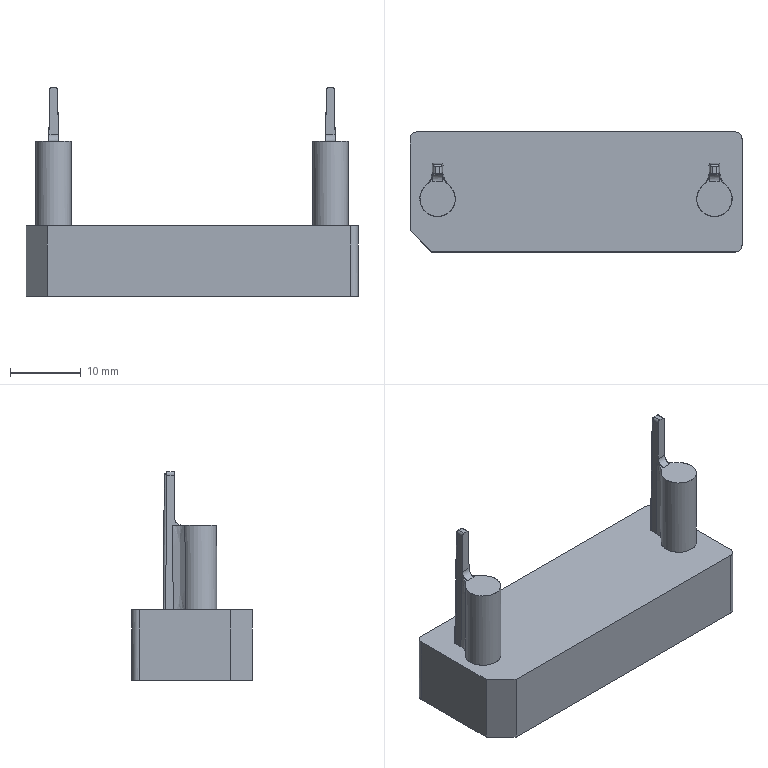NC program | PowerMill | posted with a generic post | part box 47 x 17 x 29.578 mm
Lines 10016 to 10829 of 182382:
N10113 M6
N10114 S8500 M03
N10115 G00 G90 X0.0 Y0.0
N10116 G43 Z11.798 H3
N10117
N10118 G05 P10000 R8
N10119 X-7.8085 Y4.5718
N10120 Z-6.78
N10121 G01 Z-7.98 F360.0
N10122 X-12.585 Y2.3334 F600.0
N10123 G03 X-12.6868 Y1.9988 I0.4982 J-0.3345
N10124 G01 X-12.6961 Y1.1864
N10125 X-12.7289 Y0.8046
N10126 G02 X-12.8666 Y0.0409 I-7.2156 J0.9069
N10127 G01 X-12.9741 Y-0.341
N10128 X-13.0825 Y-0.6564
N10129 X-13.2699 Y-1.1046
N10130 X-13.4635 Y-1.4865
N10131 X-13.6926 Y-1.8683
N10132 X-13.8754 Y-2.1353
N10133 X-14.0648 Y-2.3837
N10134 X-14.2757 Y-2.632
N10135 X-14.6682 Y-3.034
N10136 X-15.0918 Y-3.3957
N10137 X-15.4611 Y-3.6634
N10138 X-15.8576 Y-3.9074
N10139 X-16.3531 Y-4.1594
N10140 X-16.7 Y-4.3044
N10141 X-17.0469 Y-4.4264
N10142 X-17.4433 Y-4.5379
N10143 X-17.8398 Y-4.6218
N10144 X-18.2362 Y-4.6794
N10145 X-18.6326 Y-4.7112
N10146 X-19.0291 Y-4.7179
N10147 X-19.4255 Y-4.7001
N10148 X-20.2184 Y-4.7187
N10149 X-20.6148 Y-4.7083
N10150 X-21.0113 Y-4.6732
N10151 X-21.4077 Y-4.612
N10152 X-21.8041 Y-4.5248
N10153 X-22.2006 Y-4.4091
N10154 X-22.597 Y-4.2645
N10155 X-22.8425 Y-4.1594
N10156 X-23.3899 Y-3.8775
N10157 X-23.7469 Y-3.6541
N10158 X-24.1828 Y-3.333
N10159 X-24.5513 Y-3.0108
N10160 X-24.9757 Y-2.5686
N10161 X-25.2581 Y-2.2185
N10162 X-25.503 Y-1.8683
N10163 X-25.7685 Y-1.4179
N10164 X-25.9249 Y-1.1046
N10165 X-26.0874 Y-0.7228
N10166 X-26.2215 Y-0.341
N10167 X-26.3282 Y0.0409
N10168 X-26.4089 Y0.4227
N10169 X-26.4659 Y0.8046
N10170 X-26.4987 Y1.1864
N10171 X-26.5137 Y2.414
N10172 X-26.5306 Y2.4948
N10173 G00 Z3.9981
N10174 G01 X-19.1136 Y-9.0107 F10000.0
N10175 G00 Z0.7981
N10176 G01 Z-0.4019 F360.0
N10177 X-19.147 Y-3.7358 F600.0
N10178 Y0.5589
N10179 G03 X-17.8411 Y1.8648 I0.0 J1.3059
N10180 G03 X-20.4529 I-1.3059 J0.0
N10181 G03 X-19.147 Y0.5589 I1.3059 J0.0
N10182 G01 Y-3.7358
N10183 G00 Z5.6117
N10184 G01 X31.4193 Y4.5014 F10000.0
N10185 G00 Z-6.78
N10186 G01 Z-7.98 F360.0
N10187 X26.616 Y2.3211 F600.0
N10188 G03 X26.508 Y1.9777 I0.492 J-0.3434
N10189 G01 X26.4987 Y1.1864
N10190 X26.4662 Y0.8046
N10191 X26.4089 Y0.4227
N10192 X26.3278 Y0.0409
N10193 X26.2215 Y-0.341
N10194 X26.0874 Y-0.7228
N10195 X25.9249 Y-1.1046
N10196 X25.7685 Y-1.4179
N10197 X25.503 Y-1.8683
N10198 X25.2581 Y-2.2185
N10199 X24.9199 Y-2.632
N10200 X24.5513 Y-3.0108
N10201 X24.1038 Y-3.3957
N10202 X23.7469 Y-3.6541
N10203 X23.3899 Y-3.8775
N10204 X22.8425 Y-4.1594
N10205 X22.597 Y-4.2645
N10206 X22.2006 Y-4.4091
N10207 X21.8041 Y-4.5248
N10208 X21.4077 Y-4.612
N10209 X21.0113 Y-4.6732
N10210 X20.6148 Y-4.7083
N10211 X20.2184 Y-4.7187
N10212 X19.4255 Y-4.7001
N10213 X19.0291 Y-4.7179
N10214 X18.6326 Y-4.7112
N10215 X18.2362 Y-4.6794
N10216 X17.8398 Y-4.6218
N10217 X17.4433 Y-4.5379
N10218 X17.0469 Y-4.4264
N10219 X16.7 Y-4.3044
N10220 X16.254 Y-4.1139
N10221 X15.8576 Y-3.9074
N10222 X15.4611 Y-3.6634
N10223 X15.0918 Y-3.3957
N10224 X14.6682 Y-3.034
N10225 X14.2757 Y-2.632
N10226 X14.0648 Y-2.3837
N10227 X13.8754 Y-2.1353
N10228 X13.6926 Y-1.8683
N10229 X13.4633 Y-1.4865
N10230 X13.2699 Y-1.1046
N10231 X13.0825 Y-0.6564
N10232 X12.9741 Y-0.341
N10233 X12.8672 Y0.0409
N10234 X12.7859 Y0.4227
N10235 X12.7288 Y0.8046
N10236 X12.6961 Y1.1864
N10237 X12.6818 Y2.4218
N10238 X12.6664 Y2.499
N10239 G00 Z3.9981
N10240 G01 X19.0662 Y14.103 F10000.0
N10241 G00 Z0.7981
N10242 G01 Z-0.4019 F360.0
N10243 X19.1174 Y8.8282 F600.0
N10244 Y4.566
N10245 G03 X17.7611 Y3.2097 I0.0 J-1.3563
N10246 G03 X20.4737 I1.3563 J0.0
N10247 G03 X19.1174 Y4.566 I-1.3563 J0.0
N10248 G01 Y8.8282
N10249 G00 Z11.798
N10250 G05 P0
N10251 (---------------)
N10252 ( END TOOLPATH : 粗公基准台01-平坦面偏置-D10 )
N10253 (---------------)
N10254 ( START TOOLPATH : 粗公基准台01-基准面偏置-D10 )
N10255 (---------------)
N10256 G00 X0.0 Y0.0 Z9.7981
N10257 G05 P10000 R8
N10258 X34.035 Y-0.9466
N10259 Z-18.58
N10260 G01 Z-19.78 F360.0
N10261 X28.76 F600.0
N10262 X27.3406 Y-0.9827
N10263 X27.3456 Y-1.1792
N10264 X27.2856 Y-1.9654
N10265 X27.1818 Y-2.5788
N10266 X27.1433 Y-2.7515
N10267 X26.9148 Y-3.5376
N10268 X26.7644 Y-3.9307
N10269 X26.5916 Y-4.3238
N10270 X26.3939 Y-4.7084
N10271 X26.1577 Y-5.1099
N10272 X25.8999 Y-5.4942
N10273 X25.5922 Y-5.8961
N10274 X25.2434 Y-6.2891
N10275 X24.8181 Y-6.7122
N10276 X24.4242 Y-7.0479
N10277 X24.0302 Y-7.3409
N10278 X23.8417 Y-7.4684
N10279 X23.2424 Y-7.8238
N10280 X22.8484 Y-8.0197
N10281 X22.4545 Y-8.1885
N10282 X22.2791 Y-8.2545
N10283 X21.6666 Y-8.4526
N10284 X21.2727 Y-8.5502
N10285 X20.8787 Y-8.6268
N10286 X20.4848 Y-8.6832
N10287 X20.0909 Y-8.719
N10288 X19.6969 Y-8.7333
N10289 X19.303 Y-8.7267
N10290 X18.909 Y-8.7036
N10291 X18.5151 Y-8.6576
N10292 X18.1212 Y-8.5924
N10293 X17.7272 Y-8.5055
N10294 X17.3333 Y-8.3955
N10295 X16.9155 Y-8.2545
N10296 X16.5335 Y-8.101
N10297 X16.1515 Y-7.9259
N10298 X15.7575 Y-7.7152
N10299 X15.3528 Y-7.4684
N10300 X14.9643 Y-7.1962
N10301 X14.5757 Y-6.8841
N10302 X14.3441 Y-6.6822
N10303 X14.0524 Y-6.3974
N10304 X13.7878 Y-6.1126
N10305 X13.6032 Y-5.8961
N10306 X13.3017 Y-5.503
N10307 X13.0369 Y-5.1099
N10308 X12.789 Y-4.6862
N10309 X12.6037 Y-4.3238
N10310 X12.4309 Y-3.9307
N10311 X12.2798 Y-3.5376
N10312 X12.2121 Y-3.3311
N10313 X12.0513 Y-2.7515
N10314 X11.9097 Y-1.9654
N10315 X11.8497 Y-1.1792
N10316 X11.8697 Y-0.3931
N10317 X11.9098 Y0.0
N10318 X11.9705 Y0.3931
N10319 X12.1552 Y1.1792
N10320 X12.2121 Y1.3642
N10321 X12.4306 Y1.9654
N10322 X12.513 Y2.1692
N10323 G03 X12.5857 Y2.5625 I-0.9272 J0.3747
N10324 G01 X12.5822 Y3.5376
N10325 X12.6014 Y4.3238
N10326 X12.6446 Y4.7169
N10327 X12.713 Y5.1099
N10328 X12.808 Y5.503
N10329 X12.93 Y5.8961
N10330 X13.0 Y6.0872
N10331 X13.2531 Y6.6822
N10332 X13.4634 Y7.0753
N10333 X13.7109 Y7.4684
N10334 X14.048 Y7.9159
N10335 X14.3411 Y8.2545
N10336 X14.5757 Y8.4956
N10337 X14.8962 Y8.7867
N10338 X15.2166 Y9.0406
N10339 X15.3636 Y9.1466
N10340 X15.7575 Y9.3994
N10341 X16.1515 Y9.6195
N10342 X16.5931 Y9.8268
N10343 X16.9394 Y9.9611
N10344 X17.3333 Y10.0861
N10345 X17.7272 Y10.1838
N10346 X18.1212 Y10.2565
N10347 X18.5151 Y10.3082
N10348 X18.909 Y10.3341
N10349 X20.0909 Y10.3381
N10350 X20.4848 Y10.324
N10351 X20.8787 Y10.2851
N10352 X21.2727 Y10.2216
N10353 X21.6666 Y10.1377
N10354 X22.0606 Y10.0266
N10355 X22.4545 Y9.8867
N10356 X22.9219 Y9.6805
N10357 X23.2424 Y9.512
N10358 X23.6105 Y9.293
N10359 X24.0302 Y9.0023
N10360 X24.4242 Y8.6773
N10361 X24.8535 Y8.2545
N10362 X25.1915 Y7.8614
N10363 X25.4837 Y7.4684
N10364 X25.606 Y7.2826
N10365 X25.7846 Y6.9824
N10366 X25.9415 Y6.6822
N10367 X26.1168 Y6.2891
N10368 X26.2646 Y5.8961
N10369 X26.3939 Y5.4777
N10370 X26.4824 Y5.1099
N10371 X26.5506 Y4.7169
N10372 X26.5939 Y4.3238
N10373 X26.6132 Y3.5376
N10374 X26.6119 Y2.547
N10375 G03 X26.6943 Y2.1276 I0.9997 J-0.0213
N10376 G01 X26.7647 Y1.9654
N10377 X27.0394 Y1.1792
N10378 G02 X27.2241 Y0.3931 I-7.7339 J-2.2314
N10379 G01 X27.3256 Y-0.3931
N10380 X27.3406 Y-0.9827
N10381 X28.76 Y-0.9466
N10382 G00 Z2.8214
N10383 G01 X-34.0345 Y-1.1435 F10000.0
N10384 G00 Z-18.58
N10385 G01 Z-19.78 F360.0
N10386 X-28.7595 Y-1.1432 F600.0
N10387 X-27.3456 Y-1.1792
N10388 X-27.3256 Y-0.3931
N10389 X-27.2241 Y0.3931
N10390 X-27.1398 Y0.788
N10391 X-27.0394 Y1.1792
N10392 X-26.7647 Y1.9654
N10393 X-26.6824 Y2.1688
N10394 G03 X-26.6096 Y2.563 I-0.9269 J0.3751
N10395 G01 X-26.6132 Y3.5376
N10396 X-26.5939 Y4.3238
N10397 X-26.5503 Y4.7169
N10398 X-26.4824 Y5.1099
N10399 X-26.3939 Y5.4777
N10400 X-26.2646 Y5.8961
N10401 X-26.1172 Y6.2891
N10402 X-25.9415 Y6.6822
N10403 X-25.7847 Y6.9824
N10404 X-25.606 Y7.2826
N10405 X-25.4837 Y7.4684
N10406 X-25.1918 Y7.8614
N10407 X-24.8181 Y8.2929
N10408 X-24.4242 Y8.6773
N10409 X-23.9787 Y9.0406
N10410 X-23.6105 Y9.293
N10411 X-23.2424 Y9.512
N10412 X-22.9219 Y9.6805
N10413 X-22.4545 Y9.8867
N10414 X-22.0606 Y10.0266
N10415 X-21.6666 Y10.1377
N10416 X-21.2727 Y10.2216
N10417 X-20.8787 Y10.2851
N10418 X-20.4848 Y10.324
N10419 X-20.0909 Y10.3381
N10420 X-18.909 Y10.3341
N10421 X-18.5151 Y10.3082
N10422 X-18.1212 Y10.2565
N10423 X-17.7272 Y10.1838
N10424 X-17.3333 Y10.0861
N10425 X-16.9394 Y9.9611
N10426 X-16.5931 Y9.8268
N10427 X-16.1515 Y9.6195
N10428 X-15.7575 Y9.3994
N10429 X-15.3636 Y9.1466
N10430 X-15.2166 Y9.0406
N10431 X-14.8962 Y8.7867
N10432 X-14.5757 Y8.4956
N10433 X-14.3411 Y8.2545
N10434 X-14.0477 Y7.9159
N10435 X-13.7109 Y7.4684
N10436 X-13.4632 Y7.0753
N10437 X-13.2531 Y6.6822
N10438 X-13.0 Y6.0872
N10439 X-12.93 Y5.8961
N10440 X-12.8077 Y5.503
N10441 X-12.713 Y5.1099
N10442 X-12.6445 Y4.7169
N10443 X-12.6014 Y4.3238
N10444 X-12.5822 Y3.5376
N10445 X-12.583 Y2.545
N10446 G03 X-12.5014 Y2.1293 I0.9998 J-0.0195
N10447 G01 X-12.4306 Y1.9654
N10448 X-12.2121 Y1.3642
N10449 X-12.1552 Y1.1792
N10450 X-11.9705 Y0.3931
N10451 X-11.869 Y-0.4193
N10452 X-2.2734 Y0.1437
N10453 G02 X-2.2792 Y-2.1608 I-18.8247 J-1.1045
N10454 G01 X-2.3297 Y-2.9522
N10455 G03 X-1.2091 Y-4.1467 I1.1208 J-0.0714
N10456 G01 X1.2114 Y-4.147
N10457 G03 X2.332 Y-2.9567 I0.0001 J1.1225
N10458 G01 X2.276 Y-2.0314
N10459 G02 X2.295 Y0.3071 I17.0305 J1.031
N10460 G01 X2.3313 Y0.7203
N10461 X2.641 Y2.8499
N10462 G03 X1.5166 Y4.1496 I-1.1244 J0.1635
N10463 G01 X-1.5162
N10464 G03 X-2.6206 Y2.825 I0.0 J-1.1226
N10465 G01 X-2.5487 Y2.4317
N10466 G02 X-2.2734 Y0.1437 I-18.5495 J-3.3925
N10467 G01 X-7.0704 Y-0.1377
N10468 G03 X-7.198 Y1.0035 I-12.6157 J-0.8323
N10469 G01 X-7.9137 Y5.5324
N10470 G03 X-8.2698 Y7.082 I-11.3678 J-1.7964
N10471 G01 X-8.4987 Y7.8355
N10472 G02 X-7.6689 Y8.9549 I0.8298 J0.2521
N10473 G01 X7.6689
N10474 G02 X8.4947 Y7.8198 I0.0 J-0.8679
N10475 G01 X8.3902 Y7.497
N10476 G03 X7.8975 Y5.4331 I12.8607 J-4.1612
N10477 G01 X7.1542 Y0.6691
N10478 X7.1051 Y0.2146
N10479 G03 X8.7248 Y-7.2436 I12.424 J-1.2068
N10480 G01 X9.0865 Y-7.8687
N10481 G02 X8.461 Y-8.9532 I-0.6254 J-0.3619
N10482 G01 X-8.4587 Y-8.951
N10483 G02 X-9.0747 Y-7.8513 I0.0001 J0.7224
N10484 G01 X-8.9039 Y-7.5725
N10485 G03 X-7.0704 Y-0.1377 I-10.7821 J6.6025
N10486 G01 X-11.869 Y-0.4193
N10487 X-11.8497 Y-1.1792
N10488 X-11.9097 Y-1.9654
N10489 X-12.0513 Y-2.7515
N10490 X-12.2121 Y-3.3311
N10491 X-12.2798 Y-3.5376
N10492 X-12.4306 Y-3.9307
N10493 X-12.6037 Y-4.3238
N10494 X-12.7884 Y-4.6862
N10495 X-13.0369 Y-5.1099
N10496 X-13.3014 Y-5.503
N10497 X-13.6032 Y-5.8961
N10498 X-13.7878 Y-6.1126
N10499 X-14.0517 Y-6.3959
N10500 X-14.3441 Y-6.6822
N10501 X-14.5757 Y-6.8872
N10502 X-14.9658 Y-7.1969
N10503 X-15.3528 Y-7.4684
N10504 X-15.7575 Y-7.7152
N10505 X-16.1515 Y-7.9259
N10506 X-16.5362 Y-8.1025
N10507 X-16.9155 Y-8.2545
N10508 X-17.3333 Y-8.3955
N10509 X-17.7272 Y-8.5055
N10510 X-18.1212 Y-8.5924
N10511 X-18.5151 Y-8.6576
N10512 X-18.909 Y-8.7036
N10513 X-19.303 Y-8.7267
N10514 X-19.6969 Y-8.7333
N10515 X-20.0909 Y-8.719
N10516 X-20.4848 Y-8.6832
N10517 X-20.8787 Y-8.6268
N10518 X-21.2727 Y-8.5502
N10519 X-21.6666 Y-8.4526
N10520 X-22.2791 Y-8.2545
N10521 X-22.4545 Y-8.1885
N10522 X-22.8484 Y-8.0197
N10523 X-23.2424 Y-7.8238
N10524 X-23.8417 Y-7.4684
N10525 X-24.0302 Y-7.3409
N10526 X-24.4242 Y-7.0479
N10527 X-24.8181 Y-6.7122
N10528 X-25.0368 Y-6.5048
N10529 X-25.2472 Y-6.2891
N10530 X-25.5922 Y-5.8961
N10531 X-25.9 Y-5.4942
N10532 X-26.1577 Y-5.1099
N10533 X-26.3939 Y-4.7084
N10534 X-26.5916 Y-4.3238
N10535 X-26.7651 Y-3.9307
N10536 X-26.9148 Y-3.5376
N10537 X-27.1433 Y-2.7515
N10538 X-27.1818 Y-2.5788
N10539 X-27.2856 Y-1.9654
N10540 X-27.3456 Y-1.1792
N10541 X-28.7595 Y-1.1432
N10542 G00 Z9.7981
N10543 G05 P0
N10544 (---------------)
N10545 ( END TOOLPATH : 粗公基准台01-基准面偏置-D10 )
N10546 (---------------)
N10547 ( START TOOLPATH : 粗公基准台01-基准台侧光-D10 )
N10548 (---------------)
N10549 G00 X0.0 Y0.0 Z9.7981
N10550 G05 P10000 R8
N10551 X28.6685 Y-16.7036
N10552 Z-28.48
N10553 G01 Z-29.68 F360.0
N10554 G03 X25.8678 Y-12.5616 I-1.4004 J2.071 F600.0
N10555 G01 X25.8378 Y-12.5819
N10556 X25.8361 Y-12.583
N10557 X25.8344 Y-12.584
N10558 X25.5196 Y-12.7745
N10559 X25.5174 Y-12.7757
N10560 X25.5152 Y-12.7769
N10561 X25.0683 Y-13.0105
N10562 X25.0651 Y-13.0121
N10563 X25.0619 Y-13.0135
N10564 X24.6149 Y-13.1993
N10565 X24.6121 Y-13.2005
N10566 X24.6091 Y-13.2015
N10567 X24.1622 Y-13.3481
N10568 X24.1592 Y-13.349
N10569 X24.1561 Y-13.3498
N10570 X23.7092 Y-13.4585
N10571 X23.707 Y-13.459
N10572 X23.7049 Y-13.4594
N10573 X23.5507 Y-13.4882
N10574 X23.5493 Y-13.4885
N10575 X23.5479 Y-13.4887
N10576 X23.2551 Y-13.5326
N10577 X23.2526 Y-13.533
N10578 X23.25 Y-13.5333
N10579 X22.803 Y-13.571
N10580 X22.8004 Y-13.5712
N10581 X22.7978
N10582 X22.3509 Y-13.58
N10583 X22.3501
N10584 X22.3493
N10585 X-20.5613 Y-13.5796
N10586 X-20.5636
N10587 X-20.5659 Y-13.5795
N10588 X-21.0129 Y-13.554
N10589 X-21.0164 Y-13.5537
N10590 X-21.02 Y-13.5532
N10591 X-21.4583 Y-13.4887
N10592 X-21.4619 Y-13.4881
N10593 X-21.4655 Y-13.4873
N10594 X-21.9211 Y-13.3771
N10595 X-21.9247 Y-13.3762
N10596 X-21.9283 Y-13.375
N10597 X-22.3753 Y-13.2211
N10598 X-22.3788 Y-13.2198
N10599 X-22.3822 Y-13.2184
N10600 X-22.7879 Y-13.0355
N10601 X-22.7916 Y-13.0338
N10602 X-22.7951 Y-13.0318
N10603 X-23.2833 Y-12.7495
N10604 X-23.2862 Y-12.7478
N10605 X-23.2891 Y-12.7459
N10606 X-23.5249 Y-12.5812
N10607 X-23.5267 Y-12.5799
N10608 X-23.5285 Y-12.5785
N10609 X-23.7396 Y-12.4129
N10610 X-23.7417 Y-12.4112
N10611 X-23.7438 Y-12.4094
N10612 X-24.0557 Y-12.128
N10613 X-24.0572 Y-12.1266
N10614 X-24.0587 Y-12.1252
N10615 X-26.7409 Y-9.4433
N10616 X-26.741 Y-9.4432
N10617 X-26.7411 Y-9.4431
N10618 X-27.1856 Y-8.9961
N10619 X-27.1868 Y-8.9948
N10620 X-27.188 Y-8.9935
N10621 X-27.3253 Y-8.8426
N10622 X-27.3268 Y-8.8409
N10623 X-27.3283 Y-8.8391
N10624 X-27.5677 Y-8.543
N10625 X-27.5695 Y-8.5407
N10626 X-27.5713 Y-8.5382
N10627 X-27.7789 Y-8.2381
N10628 X-27.7801 Y-8.2363
N10629 X-27.7813 Y-8.2345
N10630 X-27.8715 Y-8.0876
N10631 X-27.8729 Y-8.0853
N10632 X-27.8742 Y-8.0829
N10633 X-28.109 Y-7.636
N10634 X-28.1105 Y-7.633
N10635 X-28.1118 Y-7.6301
N10636 X-28.2337 Y-7.3434
N10637 X-28.2345 Y-7.3416
N10638 X-28.2351 Y-7.3398
N10639 X-28.2943 Y-7.1795
N10640 X-28.2952 Y-7.1771
N10641 X-28.2959 Y-7.1747
N10642 X-28.4294 Y-6.7277
N10643 X-28.4303 Y-6.7241
N10644 X-28.4312 Y-6.7205
N10645 X-28.5207 Y-6.2735
N10646 X-28.5213 Y-6.2699
N10647 X-28.5218 Y-6.2664
N10648 X-28.5699 Y-5.8194
N10649 X-28.5702 Y-5.816
N10650 X-28.5703 Y-5.8125
N10651 X-28.58 Y-5.3656
N10652 Y-5.3647
N10653 Y-5.3638
N10654 X-28.579 Y7.5988
N10655 Y7.6011
N10656 X-28.5789 Y7.6033
N10657 X-28.5532 Y8.0503
N10658 X-28.553 Y8.053
N10659 X-28.5527 Y8.0557
N10660 X-28.4964 Y8.5027
N10661 X-28.496 Y8.5059
N10662 X-28.4954 Y8.5091
N10663 X-28.4017 Y8.9561
N10664 X-28.4011 Y8.9589
N10665 X-28.4003 Y8.9617
N10666 X-28.2723 Y9.4087
N10667 X-28.2714 Y9.4118
N10668 X-28.2703 Y9.4148
N10669 X-28.1024 Y9.8618
N10670 X-28.1012 Y9.8649
N10671 X-28.0999 Y9.8679
N10672 X-27.8887 Y10.3148
N10673 X-27.8872 Y10.3178
N10674 X-27.8856 Y10.3208
N10675 X-27.6268 Y10.7677
N10676 X-27.625 Y10.7707
N10677 X-27.6231 Y10.7736
N10678 X-27.3316 Y11.1896
N10679 X-27.3294 Y11.1926
N10680 X-27.3271 Y11.1955
N10681 X-26.9206 Y11.6735
N10682 X-26.9176 Y11.6768
N10683 X-26.9145 Y11.6799
N10684 X-26.439 Y12.1269
N10685 X-26.4363 Y12.1294
N10686 X-26.4334 Y12.1317
N10687 X-25.9743 Y12.4893
N10688 X-25.9722 Y12.4909
N10689 X-25.97 Y12.4925
N10690 X-25.8378 Y12.5819
N10691 X-25.8361 Y12.583
N10692 X-25.8344 Y12.584
N10693 X-25.5196 Y12.7745
N10694 X-25.5174 Y12.7757
N10695 X-25.5152 Y12.7769
N10696 X-25.0683 Y13.0106
N10697 X-25.0651 Y13.0121
N10698 X-25.0619 Y13.0135
N10699 X-24.6149 Y13.1994
N10700 X-24.612 Y13.2005
N10701 X-24.6091 Y13.2015
N10702 X-24.1621 Y13.3481
N10703 X-24.1592 Y13.349
N10704 X-24.1561 Y13.3498
N10705 X-23.7091 Y13.4585
N10706 X-23.7061 Y13.4592
N10707 X-23.7031 Y13.4597
N10708 X-23.2561 Y13.5325
N10709 X-23.253 Y13.5329
N10710 X-23.25 Y13.5332
N10711 X-22.803 Y13.5709
N10712 X-22.8004 Y13.5711
N10713 X-22.7978 Y13.5712
N10714 X-22.3509 Y13.58
N10715 X-22.3501
N10716 X-22.3493
N10717 X0.0
N10718 X22.3493
N10719 X22.3501
N10720 X22.3509
N10721 X22.7978 Y13.5712
N10722 X22.8004 Y13.5711
N10723 X22.803 Y13.5709
N10724 X23.25 Y13.5332
N10725 X23.253 Y13.5329
N10726 X23.2561 Y13.5325
N10727 X23.7031 Y13.4597
N10728 X23.7061 Y13.4592
N10729 X23.7091 Y13.4585
N10730 X24.1561 Y13.3498
N10731 X24.1592 Y13.349
N10732 X24.1621 Y13.3481
N10733 X24.6091 Y13.2015
N10734 X24.6119 Y13.2005
N10735 X24.6146 Y13.1995
N10736 X25.011 Y13.0366
N10737 X25.0142 Y13.0352
N10738 X25.0173 Y13.0337
N10739 X25.5148 Y12.7771
N10740 X25.5172 Y12.7758
N10741 X25.5196 Y12.7745
N10742 X25.8344 Y12.584
N10743 X25.8361 Y12.583
N10744 X25.8378 Y12.5819
N10745 X25.97 Y12.4925
N10746 X25.9721 Y12.491
N10747 X25.9743 Y12.4894
N10748 X26.4212 Y12.142
N10749 X26.4239 Y12.1398
N10750 X26.4265 Y12.1375
N10751 X26.8735 Y11.7232
N10752 X26.8767 Y11.72
N10753 X26.8797 Y11.7168
N10754 X27.3025 Y11.2269
N10755 X27.305 Y11.2239
N10756 X27.3073 Y11.2208
N10757 X27.6229 Y10.7738
N10758 X27.6249 Y10.7708
N10759 X27.6268 Y10.7677
N10760 X27.8856 Y10.3208
N10761 X27.8872 Y10.3178
N10762 X27.8887 Y10.3148
N10763 X28.0999 Y9.8679
N10764 X28.1011 Y9.8651
N10765 X28.1022 Y9.8623
N10766 X28.2348 Y9.5166
N10767 X28.2358 Y9.5138
N10768 X28.2368 Y9.5108
N10769 X28.4001 Y8.9626
N10770 X28.401 Y8.9594
N10771 X28.4017 Y8.9561
N10772 X28.4954 Y8.5091
N10773 X28.496 Y8.5059
N10774 X28.4964 Y8.5027
N10775 X28.5528 Y8.0557
N10776 X28.5531 Y8.053
N10777 X28.5533 Y8.0503
N10778 X28.5789 Y7.6033
N10779 X28.579 Y7.601
N10780 X28.5791 Y7.5988
N10781 X28.579 Y-7.5988
N10782 Y-7.6011
N10783 X28.5789 Y-7.6033
N10784 X28.5532 Y-8.0503
N10785 X28.553 Y-8.053
N10786 X28.5527 Y-8.0557
N10787 X28.4964 Y-8.5027
N10788 X28.496 Y-8.5059
N10789 X28.4954 Y-8.5091
N10790 X28.4017 Y-8.9561
N10791 X28.4011 Y-8.9589
N10792 X28.4003 Y-8.9617
N10793 X28.2723 Y-9.4087
N10794 X28.2714 Y-9.4118
N10795 X28.2703 Y-9.4148
N10796 X28.1024 Y-9.8618
N10797 X28.1012 Y-9.8649
N10798 X28.0999 Y-9.8679
N10799 X27.8887 Y-10.3148
N10800 X27.8872 Y-10.3178
N10801 X27.8856 Y-10.3208
N10802 X27.6268 Y-10.7677
N10803 X27.625 Y-10.7707
N10804 X27.6231 Y-10.7736
N10805 X27.3316 Y-11.1896
N10806 X27.3294 Y-11.1926
N10807 X27.3271 Y-11.1955
N10808 X26.9206 Y-11.6735
N10809 X26.9176 Y-11.6768
N10810 X26.9145 Y-11.6799
N10811 X26.439 Y-12.1269
N10812 X26.4363 Y-12.1294
N10813 X26.4334 Y-12.1317
N10814 X25.9743 Y-12.4893
N10815 X25.9722 Y-12.4909
N10816 X25.97 Y-12.4925
N10817 X25.8678 Y-12.5616
N10818 G03 X28.6685 Y-16.7036 I1.4003 J-2.071
N10819 G01 X28.6178 Y-16.6413
N10820 G03 X25.8171 Y-12.4992 I-1.4003 J2.071
N10821 G01 X25.793 Y-12.5156
N10822 X25.4782 Y-12.706
N10823 X25.0312 Y-12.9396
N10824 X24.5842 Y-13.1255
N10825 X24.1372 Y-13.272
N10826 X23.6902 Y-13.3808
N10827 X23.536 Y-13.4096
N10828 X23.2433 Y-13.4535
N10829 X22.7963 Y-13.4913
N10830 X22.3493 Y-13.5
N10831 X-20.5613 Y-13.4996
N10832 X-21.0083 Y-13.4741
N10833 X-21.4467 Y-13.4096
N10834 X-21.9023 Y-13.2994
N10835 X-22.3493 Y-13.1454
N10836 X-22.7551 Y-12.9626
N10837 X-23.2433 Y-12.6803
N10838 X-23.4791 Y-12.5156
N10839 X-23.6902 Y-12.35
N10840 X-24.0021 Y-12.0686
N10841 X-26.6844 Y-9.3867
N10842 X-27.1289 Y-8.9397
N10843 X-27.2661 Y-8.7888
N10844 X-27.5055 Y-8.4927
N10845 X-27.7131 Y-8.1926
N10846 X-27.8034 Y-8.0457
N10847 X-28.0382 Y-7.5988
N10848 X-28.1601 Y-7.3121
N10849 X-28.2193 Y-7.1518
N10850 X-28.3527 Y-6.7048
N10851 X-28.4422 Y-6.2578
N10852 X-28.4903 Y-5.8108
N10853 X-28.5 Y-5.3638
N10854 X-28.499 Y7.5988
N10855 X-28.4734 Y8.0457
N10856 X-28.4171 Y8.4927
N10857 X-28.3234 Y8.9397
N10858 X-28.1954 Y9.3867
N10859 X-28.0275 Y9.8337
N10860 X-27.8163 Y10.2807
N10861 X-27.5576 Y10.7277
N10862 X-27.2661 Y11.1437
N10863 X-26.8597 Y11.6216
N10864 X-26.3842 Y12.0686
N10865 X-25.9252 Y12.4262
N10866 X-25.793 Y12.5156
N10867 X-25.4782 Y12.706
N10868 X-25.0312 Y12.9397
N10869 X-24.5842 Y13.1255
N10870 X-24.1372 Y13.2721
N10871 X-23.6902 Y13.3808
N10872 X-23.2433 Y13.4535
N10873 X-22.7963 Y13.4912
N10874 X-22.3493 Y13.5
N10875 X0.0
N10876 X22.3493
N10877 X22.7963 Y13.4912
N10878 X23.2433 Y13.4535
N10879 X23.6902 Y13.3808
N10880 X24.1372 Y13.2721
N10881 X24.5842 Y13.1255
N10882 X24.9806 Y12.9626
N10883 X25.4782 Y12.706
N10884 X25.793 Y12.5156
N10885 X25.9252 Y12.4262
N10886 X26.3722 Y12.0789
N10887 X26.8191 Y11.6645
N10888 X27.2419 Y11.1746
N10889 X27.5576 Y10.7277
N10890 X27.8163 Y10.2807
N10891 X28.0275 Y9.8337
N10892 X28.1601 Y9.488
N10893 X28.3234 Y8.9397
N10894 X28.4171 Y8.4927
N10895 X28.4734 Y8.0457
N10896 X28.4991 Y7.5988
N10897 X28.499 Y-7.5988
N10898 X28.4734 Y-8.0457
N10899 X28.4171 Y-8.4927
N10900 X28.3234 Y-8.9397
N10901 X28.1954 Y-9.3867
N10902 X28.0275 Y-9.8337
N10903 X27.8163 Y-10.2807
N10904 X27.5576 Y-10.7277
N10905 X27.2661 Y-11.1437
N10906 X26.8597 Y-11.6216
N10907 X26.3842 Y-12.0686
N10908 X25.9252 Y-12.4262
N10909 X25.8171 Y-12.4992
N10910 G03 X28.6179 Y-16.6412 I1.4004 J-2.071
N10911 G00 Z9.7981
N10912 G05 P0
N10913 (---------------)
N10914 ( END TOOLPATH : 粗公基准台01-基准台侧光-D10 )
N10915 (---------------)
N10916
N10917 M05
N10918 G53 Z0.0
N10919 (---------------)
N10920 ( START TOOLPATH : 粗公精光01-等高-D4 )
N10921 (---------------)
N10922 ( TOOL NO.    :14 )
N10923 ( TOOL TYPE   : ENDMILL)
N10924 ( TOOL ID     : D4_2_1)
N10925 ( TOOL DIA    : 4.0 LENGTH 74.6)
N10926 T14